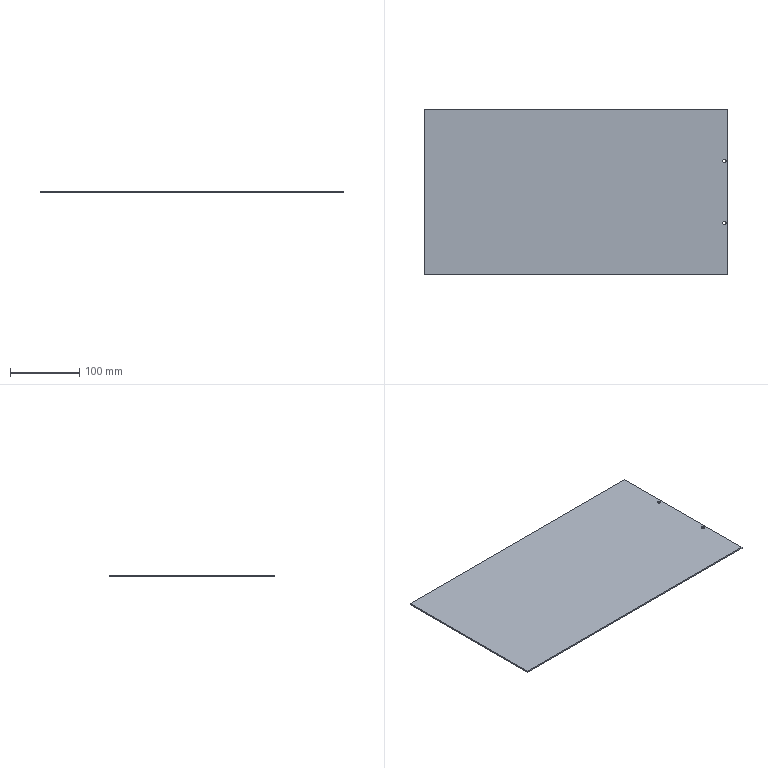Part | SolidWorks | features Cut 1, Extrusion 1 | 1 solid | 10 faces | box 440 x 240 x 2 mm | volume 211121 mm3 | plane 6 | cylinder 4 | commonest cylinder face diameters 5 x4
STEP:
#1=CARTESIAN_POINT('',(212.5,44.997,0.));
#2=VERTEX_POINT('',#1);
#3=CARTESIAN_POINT('',(217.5,44.997,0.));
#4=VERTEX_POINT('',#3);
#5=CARTESIAN_POINT('',(215.,44.997,0.));
#6=DIRECTION('',(0.,0.,1.));
#7=DIRECTION('',(1.,0.,0.));
#8=AXIS2_PLACEMENT_3D('',#5,#6,#7);
#9=CIRCLE('',#8,2.5);
#10=EDGE_CURVE('',#2,#4,#9,.T.);
#11=ORIENTED_EDGE('',*,*,#10,.F.);
#12=CARTESIAN_POINT('',(212.5,44.997,2.));
#13=VERTEX_POINT('',#12);
#14=CARTESIAN_POINT('',(212.5,44.997,0.));
#15=DIRECTION('',(0.,0.,1.));
#16=VECTOR('',#15,1000.);
#17=LINE('',#14,#16);
#18=EDGE_CURVE('',#2,#13,#17,.T.);
#19=ORIENTED_EDGE('',*,*,#18,.T.);
#20=CARTESIAN_POINT('',(217.5,44.997,2.));
#21=VERTEX_POINT('',#20);
#22=CARTESIAN_POINT('',(215.,44.997,2.));
#23=DIRECTION('',(0.,0.,1.));
#24=DIRECTION('',(1.,0.,0.));
#25=AXIS2_PLACEMENT_3D('',#22,#23,#24);
#26=CIRCLE('',#25,2.5);
#27=EDGE_CURVE('',#13,#21,#26,.T.);
#28=ORIENTED_EDGE('',*,*,#27,.T.);
#29=CARTESIAN_POINT('',(217.5,44.997,0.));
#30=DIRECTION('',(0.,0.,1.));
#31=VECTOR('',#30,1000.);
#32=LINE('',#29,#31);
#33=EDGE_CURVE('',#4,#21,#32,.T.);
#34=ORIENTED_EDGE('',*,*,#33,.F.);
#35=EDGE_LOOP('',(#11,#19,#28,#34));
#36=FACE_OUTER_BOUND('',#35,.T.);
#37=CARTESIAN_POINT('',(215.,44.997,0.));
#38=DIRECTION('',(0.,0.,1.));
#39=DIRECTION('',(1.,0.,0.));
#40=AXIS2_PLACEMENT_3D('',#37,#38,#39);
#41=CYLINDRICAL_SURFACE('',#40,2.5);
#42=ADVANCED_FACE('',(#36),#41,.F.);
#43=CARTESIAN_POINT('',(212.5,-45.003,0.));
#44=VERTEX_POINT('',#43);
#45=CARTESIAN_POINT('',(217.5,-45.003,0.));
#46=VERTEX_POINT('',#45);
#47=CARTESIAN_POINT('',(215.,-45.003,0.));
#48=DIRECTION('',(0.,0.,1.));
#49=DIRECTION('',(1.,0.,0.));
#50=AXIS2_PLACEMENT_3D('',#47,#48,#49);
#51=CIRCLE('',#50,2.5);
#52=EDGE_CURVE('',#44,#46,#51,.T.);
#53=ORIENTED_EDGE('',*,*,#52,.F.);
#54=CARTESIAN_POINT('',(212.5,-45.003,2.));
#55=VERTEX_POINT('',#54);
#56=CARTESIAN_POINT('',(212.5,-45.003,0.));
#57=DIRECTION('',(0.,0.,1.));
#58=VECTOR('',#57,1000.);
#59=LINE('',#56,#58);
#60=EDGE_CURVE('',#44,#55,#59,.T.);
#61=ORIENTED_EDGE('',*,*,#60,.T.);
#62=CARTESIAN_POINT('',(217.5,-45.003,2.));
#63=VERTEX_POINT('',#62);
#64=CARTESIAN_POINT('',(215.,-45.003,2.));
#65=DIRECTION('',(0.,0.,1.));
#66=DIRECTION('',(1.,0.,0.));
#67=AXIS2_PLACEMENT_3D('',#64,#65,#66);
#68=CIRCLE('',#67,2.5);
#69=EDGE_CURVE('',#55,#63,#68,.T.);
#70=ORIENTED_EDGE('',*,*,#69,.T.);
#71=CARTESIAN_POINT('',(217.5,-45.003,0.));
#72=DIRECTION('',(0.,0.,1.));
#73=VECTOR('',#72,1000.);
#74=LINE('',#71,#73);
#75=EDGE_CURVE('',#46,#63,#74,.T.);
#76=ORIENTED_EDGE('',*,*,#75,.F.);
#77=EDGE_LOOP('',(#53,#61,#70,#76));
#78=FACE_OUTER_BOUND('',#77,.T.);
#79=CARTESIAN_POINT('',(215.,-45.003,0.));
#80=DIRECTION('',(0.,0.,1.));
#81=DIRECTION('',(1.,0.,0.));
#82=AXIS2_PLACEMENT_3D('',#79,#80,#81);
#83=CYLINDRICAL_SURFACE('',#82,2.5);
#84=ADVANCED_FACE('',(#78),#83,.F.);
#85=CARTESIAN_POINT('',(220.,-120.,0.));
#86=VERTEX_POINT('',#85);
#87=CARTESIAN_POINT('',(220.,120.,0.));
#88=VERTEX_POINT('',#87);
#89=CARTESIAN_POINT('',(220.,120.,0.));
#90=DIRECTION('',(0.,1.,0.));
#91=VECTOR('',#90,1000.);
#92=LINE('',#89,#91);
#93=EDGE_CURVE('',#86,#88,#92,.T.);
#94=ORIENTED_EDGE('',*,*,#93,.T.);
#95=CARTESIAN_POINT('',(220.,120.,2.));
#96=VERTEX_POINT('',#95);
#97=CARTESIAN_POINT('',(220.,120.,2.));
#98=DIRECTION('',(0.,0.,-1.));
#99=VECTOR('',#98,1000.);
#100=LINE('',#97,#99);
#101=EDGE_CURVE('',#96,#88,#100,.T.);
#102=ORIENTED_EDGE('',*,*,#101,.F.);
#103=CARTESIAN_POINT('',(220.,-120.,2.));
#104=VERTEX_POINT('',#103);
#105=CARTESIAN_POINT('',(220.,120.,2.));
#106=DIRECTION('',(0.,1.,0.));
#107=VECTOR('',#106,1000.);
#108=LINE('',#105,#107);
#109=EDGE_CURVE('',#104,#96,#108,.T.);
#110=ORIENTED_EDGE('',*,*,#109,.F.);
#111=CARTESIAN_POINT('',(220.,-120.,2.));
#112=DIRECTION('',(0.,0.,-1.));
#113=VECTOR('',#112,1000.);
#114=LINE('',#111,#113);
#115=EDGE_CURVE('',#104,#86,#114,.T.);
#116=ORIENTED_EDGE('',*,*,#115,.T.);
#117=EDGE_LOOP('',(#94,#102,#110,#116));
#118=FACE_OUTER_BOUND('',#117,.T.);
#119=CARTESIAN_POINT('',(220.,120.,2.));
#120=DIRECTION('',(-1.,0.,0.));
#121=DIRECTION('',(0.,0.,1.));
#122=AXIS2_PLACEMENT_3D('',#119,#120,#121);
#123=PLANE('',#122);
#124=ADVANCED_FACE('',(#118),#123,.F.);
#125=CARTESIAN_POINT('',(-220.,120.,0.));
#126=VERTEX_POINT('',#125);
#127=CARTESIAN_POINT('',(-220.,120.,0.));
#128=DIRECTION('',(-1.,0.,0.));
#129=VECTOR('',#128,1000.);
#130=LINE('',#127,#129);
#131=EDGE_CURVE('',#88,#126,#130,.T.);
#132=ORIENTED_EDGE('',*,*,#131,.T.);
#133=CARTESIAN_POINT('',(-220.,120.,2.));
#134=VERTEX_POINT('',#133);
#135=CARTESIAN_POINT('',(-220.,120.,2.));
#136=DIRECTION('',(0.,0.,-1.));
#137=VECTOR('',#136,1000.);
#138=LINE('',#135,#137);
#139=EDGE_CURVE('',#134,#126,#138,.T.);
#140=ORIENTED_EDGE('',*,*,#139,.F.);
#141=CARTESIAN_POINT('',(-220.,120.,2.));
#142=DIRECTION('',(-1.,0.,0.));
#143=VECTOR('',#142,1000.);
#144=LINE('',#141,#143);
#145=EDGE_CURVE('',#96,#134,#144,.T.);
#146=ORIENTED_EDGE('',*,*,#145,.F.);
#147=ORIENTED_EDGE('',*,*,#101,.T.);
#148=EDGE_LOOP('',(#132,#140,#146,#147));
#149=FACE_OUTER_BOUND('',#148,.T.);
#150=CARTESIAN_POINT('',(-220.,120.,2.));
#151=DIRECTION('',(0.,-1.,0.));
#152=DIRECTION('',(0.,0.,-1.));
#153=AXIS2_PLACEMENT_3D('',#150,#151,#152);
#154=PLANE('',#153);
#155=ADVANCED_FACE('',(#149),#154,.F.);
#156=CARTESIAN_POINT('',(-220.,-120.,0.));
#157=VERTEX_POINT('',#156);
#158=CARTESIAN_POINT('',(-220.,120.,0.));
#159=DIRECTION('',(0.,-1.,0.));
#160=VECTOR('',#159,1000.);
#161=LINE('',#158,#160);
#162=EDGE_CURVE('',#126,#157,#161,.T.);
#163=ORIENTED_EDGE('',*,*,#162,.T.);
#164=CARTESIAN_POINT('',(-220.,-120.,2.));
#165=VERTEX_POINT('',#164);
#166=CARTESIAN_POINT('',(-220.,-120.,2.));
#167=DIRECTION('',(0.,0.,-1.));
#168=VECTOR('',#167,1000.);
#169=LINE('',#166,#168);
#170=EDGE_CURVE('',#165,#157,#169,.T.);
#171=ORIENTED_EDGE('',*,*,#170,.F.);
#172=CARTESIAN_POINT('',(-220.,120.,2.));
#173=DIRECTION('',(0.,-1.,0.));
#174=VECTOR('',#173,1000.);
#175=LINE('',#172,#174);
#176=EDGE_CURVE('',#134,#165,#175,.T.);
#177=ORIENTED_EDGE('',*,*,#176,.F.);
#178=ORIENTED_EDGE('',*,*,#139,.T.);
#179=EDGE_LOOP('',(#163,#171,#177,#178));
#180=FACE_OUTER_BOUND('',#179,.T.);
#181=CARTESIAN_POINT('',(-220.,120.,2.));
#182=DIRECTION('',(1.,0.,0.));
#183=DIRECTION('',(0.,0.,-1.));
#184=AXIS2_PLACEMENT_3D('',#181,#182,#183);
#185=PLANE('',#184);
#186=ADVANCED_FACE('',(#180),#185,.F.);
#187=CARTESIAN_POINT('',(-220.,-120.,0.));
#188=DIRECTION('',(1.,0.,0.));
#189=VECTOR('',#188,1000.);
#190=LINE('',#187,#189);
#191=EDGE_CURVE('',#157,#86,#190,.T.);
#192=ORIENTED_EDGE('',*,*,#191,.T.);
#193=ORIENTED_EDGE('',*,*,#115,.F.);
#194=CARTESIAN_POINT('',(-220.,-120.,2.));
#195=DIRECTION('',(1.,0.,0.));
#196=VECTOR('',#195,1000.);
#197=LINE('',#194,#196);
#198=EDGE_CURVE('',#165,#104,#197,.T.);
#199=ORIENTED_EDGE('',*,*,#198,.F.);
#200=ORIENTED_EDGE('',*,*,#170,.T.);
#201=EDGE_LOOP('',(#192,#193,#199,#200));
#202=FACE_OUTER_BOUND('',#201,.T.);
#203=CARTESIAN_POINT('',(-220.,-120.,2.));
#204=DIRECTION('',(0.,1.,0.));
#205=DIRECTION('',(0.,0.,1.));
#206=AXIS2_PLACEMENT_3D('',#203,#204,#205);
#207=PLANE('',#206);
#208=ADVANCED_FACE('',(#202),#207,.F.);
#209=CARTESIAN_POINT('',(215.,44.997,2.));
#210=DIRECTION('',(0.,0.,1.));
#211=DIRECTION('',(1.,0.,0.));
#212=AXIS2_PLACEMENT_3D('',#209,#210,#211);
#213=CIRCLE('',#212,2.5);
#214=EDGE_CURVE('',#21,#13,#213,.T.);
#215=ORIENTED_EDGE('',*,*,#214,.F.);
#216=ORIENTED_EDGE('',*,*,#27,.F.);
#217=EDGE_LOOP('',(#215,#216));
#218=FACE_BOUND('',#217,.T.);
#219=CARTESIAN_POINT('',(215.,-45.003,2.));
#220=DIRECTION('',(0.,0.,1.));
#221=DIRECTION('',(1.,0.,0.));
#222=AXIS2_PLACEMENT_3D('',#219,#220,#221);
#223=CIRCLE('',#222,2.5);
#224=EDGE_CURVE('',#63,#55,#223,.T.);
#225=ORIENTED_EDGE('',*,*,#224,.F.);
#226=ORIENTED_EDGE('',*,*,#69,.F.);
#227=EDGE_LOOP('',(#225,#226));
#228=FACE_BOUND('',#227,.T.);
#229=ORIENTED_EDGE('',*,*,#109,.T.);
#230=ORIENTED_EDGE('',*,*,#145,.T.);
#231=ORIENTED_EDGE('',*,*,#176,.T.);
#232=ORIENTED_EDGE('',*,*,#198,.T.);
#233=EDGE_LOOP('',(#229,#230,#231,#232));
#234=FACE_OUTER_BOUND('',#233,.T.);
#235=CARTESIAN_POINT('',(0.,0.,2.));
#236=DIRECTION('',(0.,0.,1.));
#237=DIRECTION('',(1.,0.,0.));
#238=AXIS2_PLACEMENT_3D('',#235,#236,#237);
#239=PLANE('',#238);
#240=ADVANCED_FACE('',(#218,#228,#234),#239,.T.);
#241=CARTESIAN_POINT('',(215.,44.997,0.));
#242=DIRECTION('',(0.,0.,1.));
#243=DIRECTION('',(1.,0.,0.));
#244=AXIS2_PLACEMENT_3D('',#241,#242,#243);
#245=CIRCLE('',#244,2.5);
#246=EDGE_CURVE('',#4,#2,#245,.T.);
#247=ORIENTED_EDGE('',*,*,#246,.T.);
#248=ORIENTED_EDGE('',*,*,#10,.T.);
#249=EDGE_LOOP('',(#247,#248));
#250=FACE_BOUND('',#249,.T.);
#251=CARTESIAN_POINT('',(215.,-45.003,0.));
#252=DIRECTION('',(0.,0.,1.));
#253=DIRECTION('',(1.,0.,0.));
#254=AXIS2_PLACEMENT_3D('',#251,#252,#253);
#255=CIRCLE('',#254,2.5);
#256=EDGE_CURVE('',#46,#44,#255,.T.);
#257=ORIENTED_EDGE('',*,*,#256,.T.);
#258=ORIENTED_EDGE('',*,*,#52,.T.);
#259=EDGE_LOOP('',(#257,#258));
#260=FACE_BOUND('',#259,.T.);
#261=ORIENTED_EDGE('',*,*,#93,.F.);
#262=ORIENTED_EDGE('',*,*,#191,.F.);
#263=ORIENTED_EDGE('',*,*,#162,.F.);
#264=ORIENTED_EDGE('',*,*,#131,.F.);
#265=EDGE_LOOP('',(#261,#262,#263,#264));
#266=FACE_OUTER_BOUND('',#265,.T.);
#267=CARTESIAN_POINT('',(0.,0.,0.));
#268=DIRECTION('',(0.,0.,1.));
#269=DIRECTION('',(1.,0.,0.));
#270=AXIS2_PLACEMENT_3D('',#267,#268,#269);
#271=PLANE('',#270);
#272=ADVANCED_FACE('',(#250,#260,#266),#271,.F.);
#273=ORIENTED_EDGE('',*,*,#60,.F.);
#274=ORIENTED_EDGE('',*,*,#256,.F.);
#275=ORIENTED_EDGE('',*,*,#75,.T.);
#276=ORIENTED_EDGE('',*,*,#224,.T.);
#277=EDGE_LOOP('',(#273,#274,#275,#276));
#278=FACE_OUTER_BOUND('',#277,.T.);
#279=CARTESIAN_POINT('',(215.,-45.003,0.));
#280=DIRECTION('',(0.,0.,1.));
#281=DIRECTION('',(1.,0.,0.));
#282=AXIS2_PLACEMENT_3D('',#279,#280,#281);
#283=CYLINDRICAL_SURFACE('',#282,2.5);
#284=ADVANCED_FACE('',(#278),#283,.F.);
#285=ORIENTED_EDGE('',*,*,#18,.F.);
#286=ORIENTED_EDGE('',*,*,#246,.F.);
#287=ORIENTED_EDGE('',*,*,#33,.T.);
#288=ORIENTED_EDGE('',*,*,#214,.T.);
#289=EDGE_LOOP('',(#285,#286,#287,#288));
#290=FACE_OUTER_BOUND('',#289,.T.);
#291=CARTESIAN_POINT('',(215.,44.997,0.));
#292=DIRECTION('',(0.,0.,1.));
#293=DIRECTION('',(1.,0.,0.));
#294=AXIS2_PLACEMENT_3D('',#291,#292,#293);
#295=CYLINDRICAL_SURFACE('',#294,2.5);
#296=ADVANCED_FACE('',(#290),#295,.F.);
#297=CLOSED_SHELL('',(#42,#84,#124,#155,#186,#208,#240,#272,#284,#296));
#298=MANIFOLD_SOLID_BREP('',#297);
#299=CARTESIAN_POINT('',(0.,0.,0.));
#300=DIRECTION('',(0.,0.,1.));
#301=DIRECTION('',(1.,0.,0.));
#302=AXIS2_PLACEMENT_3D('',#299,#300,#301);
#303=(LENGTH_UNIT()NAMED_UNIT(*)SI_UNIT(.MILLI.,.METRE.));
#304=UNCERTAINTY_MEASURE_WITH_UNIT(LENGTH_MEASURE(0.00001),#303,'','');
#305=(NAMED_UNIT(*)PLANE_ANGLE_UNIT()SI_UNIT($,.RADIAN.));
#306=(NAMED_UNIT(*)SI_UNIT($,.STERADIAN.)SOLID_ANGLE_UNIT());
#307=(GEOMETRIC_REPRESENTATION_CONTEXT(3)GLOBAL_UNCERTAINTY_ASSIGNED_CONTEXT((#304))GLOBAL_UNIT_ASSIGNED_CONTEXT((#303,#305,#306))REPRESENTATION_CONTEXT('',''));
#308=ADVANCED_BREP_SHAPE_REPRESENTATION('',(#298,#302),#307);